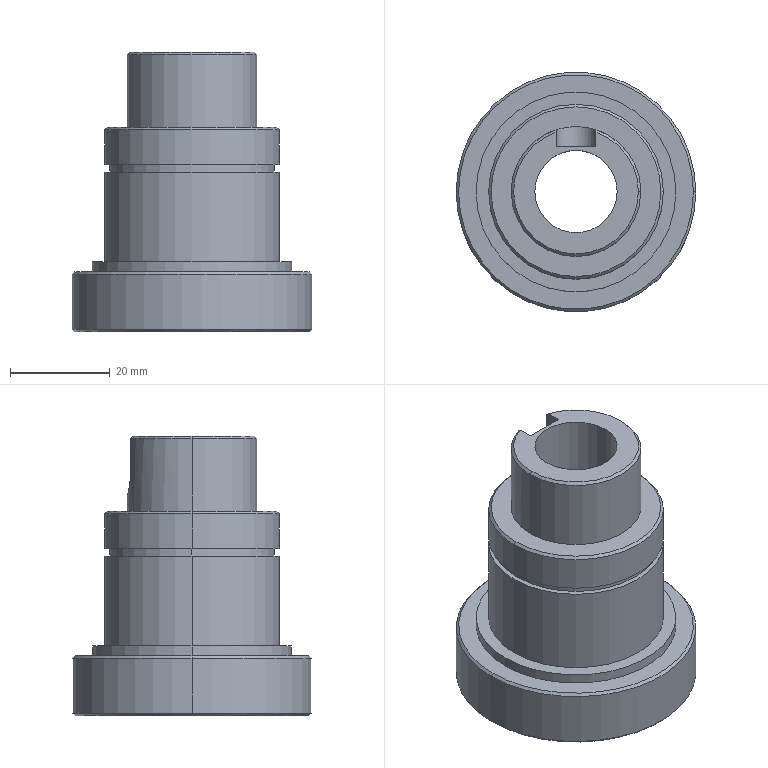Part | SolidWorks | features ICE 7, Chamfer 1, Extrusion 1, HoleWzd 1 | 1 solid | 61 faces | box 48 x 48 x 56 mm | volume 29857 mm3 | cylinder 29 | cone 21 | plane 11 | commonest cylinder face diameters 4.2 x12 35 x4 16.5 x2 26 x2 28 x2 33 x2